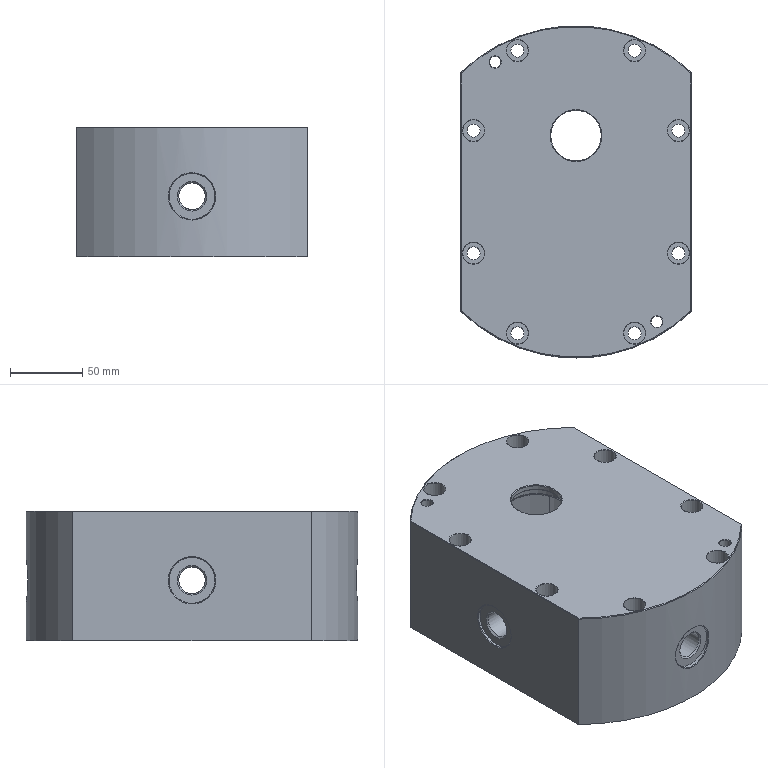NC program | NX | posted with a generic post | part box 160 x 230 x 90 mm
Lines 8806 to 9223 of 9223:
(HOLE_MILLING_COPY_COPY_COPY_COPY , TOOL : D12)
N17568 T12 M6
N17570 G54
N17572 G17 G0 G90 X43.9 Y6.945 B0. C0. S3000 M3
N17574 G43 Z30. H12
N17576 Z-77.5
N17578 G94 G3 X39. Y16.4 R5.997 F1500.
N17580 X39. Y16.4 Z-77.72 I0. J-16.4
N17582 X39. Y16.4 Z-77.94 I0. J-16.4
N17584 X39. Y16.4 Z-78.16 I0. J-16.4
N17586 X39. Y16.4 Z-78.38 I0. J-16.4
N17588 X39. Y16.4 Z-78.6 I0. J-16.4
N17590 X39. Y16.4 Z-78.82 I0. J-16.4
N17592 X39. Y16.4 Z-79.04 I0. J-16.4
N17594 X39. Y16.4 Z-79.26 I0. J-16.4
N17596 X39. Y16.4 Z-79.48 I0. J-16.4
N17598 X39. Y16.4 Z-79.7 I0. J-16.4
N17600 X39. Y16.4 Z-79.92 I0. J-16.4
N17602 X39. Y16.4 Z-80.14 I0. J-16.4
N17604 X39. Y16.4 Z-80.36 I0. J-16.4
N17606 X39. Y16.4 Z-80.58 I0. J-16.4
N17608 X39. Y16.4 Z-80.8 I0. J-16.4
N17610 X39. Y16.4 Z-81.02 I0. J-16.4
N17612 X39. Y16.4 Z-81.24 I0. J-16.4
N17614 X39. Y16.4 Z-81.46 I0. J-16.4
N17616 X39. Y16.4 Z-81.68 I0. J-16.4
N17618 X39. Y16.4 Z-81.9 I0. J-16.4
N17620 X39. Y16.4 Z-82.12 I0. J-16.4
N17622 X39. Y16.4 Z-82.34 I0. J-16.4
N17624 X39. Y16.4 Z-82.56 I0. J-16.4
N17626 X39. Y16.4 Z-82.78 I0. J-16.4
N17628 X39. Y16.4 Z-83. I0. J-16.4
N17630 X39. Y16.4 Z-83.22 I0. J-16.4
N17632 X39. Y16.4 Z-83.44 I0. J-16.4
N17634 X39. Y16.4 Z-83.66 I0. J-16.4
N17636 X39. Y16.4 Z-83.88 I0. J-16.4
N17638 X39. Y16.4 Z-84.1 I0. J-16.4
N17640 X39. Y16.4 Z-84.32 I0. J-16.4
N17642 X39. Y16.4 Z-84.54 I0. J-16.4
N17644 X39. Y16.4 Z-84.76 I0. J-16.4
N17646 X39. Y16.4 Z-84.98 I0. J-16.4
N17648 X39. Y16.4 Z-85.2 I0. J-16.4
N17650 X39. Y16.4 Z-85.42 I0. J-16.4
N17652 X39. Y16.4 Z-85.64 I0. J-16.4
N17654 X39. Y16.4 Z-85.86 I0. J-16.4
N17656 X51.394 Y-10.74 Z-86. R-16.4
N17658 X49.74 Y12.394 R16.4
N17660 X51.394 Y-10.74 R-16.4
N17662 X47.458 Y-0.845 R5.997
N17664 G0 Z30.
(FLOOR_WALL_1_COPY , TOOL : D12)
N17666 X-67.913 Y-48.287 S4000
N17668 Z-6.738
N17670 G1 Z-9.738 F500.
N17672 X-66.116 Y-51.4
N17674 G3 X-65.077 Y-52. R1.2
N17676 G1 X65.077 F1000.
N17678 G3 X72.586 Y-47.962 R9.
N17680 X72.586 Y47.962 R87.
N17682 X65.077 Y52. R9.
N17684 G1 X-65.077
N17686 G3 X-72.586 Y47.962 R9.
N17688 X-72.586 Y-47.962 R87.
N17690 X-65.077 Y-52. R9.
N17692 X-64.038 Y-51.4 R1.2
N17694 G1 X-62.652 Y-49.
N17696 Z-6.738
N17698 G0 X-67.913 Y-48.287 Z-16.475
N17700 G1 Z-19.475 F500.
N17702 X-66.116 Y-51.4
N17704 G3 X-65.077 Y-52. R1.2
N17706 G1 X65.077 F1000.
N17708 G3 X72.586 Y-47.962 R9.
N17710 X72.586 Y47.962 R87.
N17712 X65.077 Y52. R9.
N17714 G1 X-65.077
N17716 G3 X-72.586 Y47.962 R9.
N17718 X-72.586 Y-47.962 R87.
N17720 X-65.077 Y-52. R9.
N17722 X-64.038 Y-51.4 R1.2
N17724 G1 X-62.652 Y-49.
N17726 Z-16.475
N17728 G0 X-67.913 Y-48.287 Z-26.213
N17730 G1 Z-29.213 F500.
N17732 X-66.116 Y-51.4
N17734 G3 X-65.077 Y-52. R1.2
N17736 G1 X65.077 F1000.
N17738 G3 X72.586 Y-47.962 R9.
N17740 X72.586 Y47.962 R87.
N17742 X65.077 Y52. R9.
N17744 G1 X-65.077
N17746 G3 X-72.586 Y47.962 R9.
N17748 X-72.586 Y-47.962 R87.
N17750 X-65.077 Y-52. R9.
N17752 X-64.038 Y-51.4 R1.2
N17754 G1 X-62.652 Y-49.
N17756 Z-26.213
N17758 G0 X-67.913 Y-48.287 Z-35.95
N17760 G1 Z-38.95 F500.
N17762 X-66.116 Y-51.4
N17764 G3 X-65.077 Y-52. R1.2
N17766 G1 X65.077 F1000.
N17768 G3 X72.586 Y-47.962 R9.
N17770 X72.586 Y47.962 R87.
N17772 X65.077 Y52. R9.
N17774 G1 X-65.077
N17776 G3 X-72.586 Y47.962 R9.
N17778 X-72.586 Y-47.962 R87.
N17780 X-65.077 Y-52. R9.
N17782 X-64.038 Y-51.4 R1.2
N17784 G1 X-62.652 Y-49.
N17786 Z-35.95
N17788 G0 X-67.913 Y-48.287 Z-45.688
N17790 G1 Z-48.688 F500.
N17792 X-66.116 Y-51.4
N17794 G3 X-65.077 Y-52. R1.2
N17796 G1 X65.077 F1000.
N17798 G3 X72.586 Y-47.962 R9.
N17800 X72.586 Y47.962 R87.
N17802 X65.077 Y52. R9.
N17804 G1 X-65.077
N17806 G3 X-72.586 Y47.962 R9.
N17808 X-72.586 Y-47.962 R87.
N17810 X-65.077 Y-52. R9.
N17812 X-64.038 Y-51.4 R1.2
N17814 G1 X-62.652 Y-49.
N17816 Z-45.688
N17818 G0 X-67.913 Y-48.287 Z-55.425
N17820 G1 Z-58.425 F500.
N17822 X-66.116 Y-51.4
N17824 G3 X-65.077 Y-52. R1.2
N17826 G1 X65.077 F1000.
N17828 G3 X72.586 Y-47.962 R9.
N17830 X72.586 Y47.962 R87.
N17832 X65.077 Y52. R9.
N17834 G1 X-65.077
N17836 G3 X-72.586 Y47.962 R9.
N17838 X-72.586 Y-47.962 R87.
N17840 X-65.077 Y-52. R9.
N17842 X-64.038 Y-51.4 R1.2
N17844 G1 X-62.652 Y-49.
N17846 Z-55.425
N17848 G0 X-67.913 Y-48.287 Z-65.163
N17850 G1 Z-68.163 F500.
N17852 X-66.116 Y-51.4
N17854 G3 X-65.077 Y-52. R1.2
N17856 G1 X65.077 F1000.
N17858 G3 X72.586 Y-47.962 R9.
N17860 X72.586 Y47.962 R87.
N17862 X65.077 Y52. R9.
N17864 G1 X-65.077
N17866 G3 X-72.586 Y47.962 R9.
N17868 X-72.586 Y-47.962 R87.
N17870 X-65.077 Y-52. R9.
N17872 X-64.038 Y-51.4 R1.2
N17874 G1 X-62.652 Y-49.
N17876 Z-65.163
N17878 G0 X-67.913 Y-48.287 Z-74.9
N17880 G1 Z-77.9 F500.
N17882 X-66.116 Y-51.4
N17884 G3 X-65.077 Y-52. R1.2
N17886 G1 X65.077 F1000.
N17888 G3 X72.586 Y-47.962 R9.
N17890 X72.586 Y47.962 R87.
N17892 X65.077 Y52. R9.
N17894 G1 X-65.077
N17896 G3 X-72.586 Y47.962 R9.
N17898 X-72.586 Y-47.962 R87.
N17900 X-65.077 Y-52. R9.
N17902 X-64.038 Y-51.4 R1.2
N17904 G1 X-62.652 Y-49.
N17906 Z-74.9
N17908 G0 Z30.
(FLOOR_WALL_1_COPY_COPY , TOOL : D12)
N17910 X-64.167 Y50.799
N17912 Z-75.
N17914 G1 Z-78. F500.
N17916 G3 X-65.206 Y51.399 R1.2
N17918 G1 X65.206 F1000.
N17920 G2 X72.085 Y47.631 R8.4
N17922 X73.332 Y45.688 R86.4
N17924 G1 X-73.332
N17926 G3 X-76.595 Y39.977 R86.4
N17928 G1 X76.595
N17930 G2 X79.315 Y34.266 R86.4
N17932 G1 X-79.315
N17934 G3 X-81.545 Y28.555 R86.4
N17936 G1 X81.545
N17938 G2 X83.325 Y22.844 R86.4
N17940 G1 X-83.325
N17942 G3 X-84.684 Y17.133 R86.4
N17944 G1 X84.684
N17946 G2 X85.642 Y11.422 R86.4
N17948 G1 X-85.642
N17950 G3 X-86.211 Y5.711 R86.4
N17952 G1 X86.211
N17954 G2 X86.4 Y0. R86.4
N17956 G1 X-86.4
N17958 G3 X-86.211 Y-5.712 R86.4
N17960 G1 X86.211
N17962 G2 X85.642 Y-11.423 R86.4
N17964 G1 X-85.642
N17966 G3 X-84.684 Y-17.134 R86.4
N17968 G1 X84.684
N17970 G2 X83.325 Y-22.845 R86.4
N17972 G1 X-83.325
N17974 G3 X-81.545 Y-28.556 R86.4
N17976 G1 X81.545
N17978 G2 X79.314 Y-34.267 R86.4
N17980 G1 X-79.314
N17982 G3 X-76.595 Y-39.978 R86.4
N17984 G1 X76.595
N17986 G2 X73.331 Y-45.689 R86.4
N17988 G1 X-73.331
N17990 G3 X-72.085 Y-47.631 R86.4
N17992 X-65.09 Y-51.4 R8.4
N17994 G1 X65.09
N17996 G3 X66.13 Y-50.8 R1.2
N17998 G1 X64.051 Y-51.402
N18000 G3 X65.091 Y-52. R1.2 F500.
N18002 X72.586 Y-47.962 R9. F1000.
N18004 X72.586 Y47.962 R87.
N18006 X65.077 Y52. R9.
N18008 G1 X-65.077
N18010 G3 X-72.586 Y47.962 R9.
N18012 X-72.586 Y-47.962 R87.
N18014 X-65.077 Y-52. R9.
N18016 G1 X65.091
N18018 G3 X66.13 Y-51.398 R1.2
N18020 G1 X67.922 Y-48.283
N18022 Z-75.
N18024 G0 Z30.
N18026 M5
(PLANAR_MILL_COPY_COPY_COPY , TOOL : D6A45)
N18028 T07 M6
N18030 G54
N18032 G17 G0 G90 X-43.266 Y-73.843 B0. C0. S7500 M3
N18034 G43 Z30. H7
N18036 Z1.5
N18038 G94 G1 Z-1.5 F1250.
N18040 G3 X-42.5 Y-74.2 R1.
N18042 X-39.3 Y-71. R3.2
N18044 X-42.5 Y-74.2 R-3.2
N18046 X-41.734 Y-73.843 R1.
N18048 G1 Z1.5
N18050 G0 Z30.
N18052 X-100.774 Y-39.798
N18054 Z1.5
N18056 G1 Z-1.5
N18058 G3 X-101.131 Y-40.564 R1.
N18060 X-97.931 Y-43.764 R3.2
N18062 X-101.131 Y-40.564 R-3.2
N18064 X-100.774 Y-41.33 R1.
N18066 G1 Z1.5
N18068 G0 Z30.
N18070 Y41.33
N18072 Z1.5
N18074 G1 Z-1.5
N18076 G3 X-101.131 Y40.564 R1.
N18078 X-97.931 Y37.364 R3.2
N18080 X-101.131 Y40.564 R-3.2
N18082 X-100.774 Y39.798 R1.
N18084 G1 Z1.5
N18086 G0 Z30.
N18088 X-92.343 Y56.766
N18090 Z1.5
N18092 G1 Z-1.5
N18094 G3 X-92.7 Y56. R1.
N18096 X-90. Y53.3 R2.7
N18098 X-92.7 Y56. R-2.7
N18100 X-92.343 Y55.234 R1.
N18102 G1 Z1.5
N18104 G0 Z30.
N18106 X-41.734 Y73.843
N18108 Z1.5
N18110 G1 Z-1.5
N18112 G3 X-42.5 Y74.2 R1.
N18114 X-45.7 Y71. R3.2
N18116 X-42.5 Y74.2 R-3.2
N18118 X-43.266 Y73.843 R1.
N18120 G1 Z1.5
N18122 G0 Z30.
N18124 X-0.766 Y62.657
N18126 Z1.5
N18128 G1 Z-1.5
N18130 G3 X0. Y62.3 R1.
N18132 G1 X65.077
N18134 G2 X81.179 Y53.64 R19.3
N18136 X81.179 Y-53.64 R97.3
N18138 X65.077 Y-62.3 R19.3
N18140 G1 X-65.077
N18142 G2 X-81.179 Y-53.64 R19.3
N18144 X-81.179 Y53.64 R97.3
N18146 X-65.077 Y62.3 R19.3
N18148 G1 X0.
N18150 G3 X0.766 Y62.657 R1.
N18152 G1 Z1.5
N18154 G0 Z30.
N18156 Y62.343
N18158 Z1.5
N18160 G1 Z-1.5
N18162 G3 X0. Y62.7 R1.
N18164 G1 X-65.077
N18166 G3 X-81.513 Y53.86 R19.7
N18168 X-81.513 Y-53.86 R97.7
N18170 X-65.077 Y-62.7 R19.7
N18172 G1 X65.077
N18174 G3 X81.513 Y-53.86 R19.7
N18176 X81.513 Y53.86 R97.7
N18178 X65.077 Y62.7 R19.7
N18180 G1 X0.
N18182 G3 X-0.766 Y62.343 R1.
N18184 G1 Z1.5
N18186 G0 Z30.
N18188 Y81.657
N18190 Z1.5
N18192 G1 Z-1.5
N18194 G3 X0. Y81.3 R1.
N18196 G1 X82.614
N18198 G2 X83.547 Y80.904 R1.3
N18200 X83.547 Y-80.904 R116.3
N18202 X82.614 Y-81.3 R1.3
N18204 G1 X-82.614
N18206 G2 X-83.547 Y-80.904 R1.3
N18208 X-83.547 Y80.904 R116.3
N18210 X-82.614 Y81.3 R1.3
N18212 G1 X0.
N18214 G3 X0.766 Y81.657 R1.
N18216 G1 Z1.5
N18218 G0 Z30.
N18220 Y56.343
N18222 Z1.5
N18224 G1 Z-1.5
N18226 G3 X0. Y56.7 R1.
N18228 G1 X-65.077
N18230 G3 X-76.507 Y50.553 R13.7
N18232 X-76.507 Y-50.553 R91.7
N18234 X-65.077 Y-56.7 R13.7
N18236 G1 X65.077
N18238 G3 X76.507 Y-50.553 R13.7
N18240 X76.507 Y50.553 R91.7
N18242 X65.077 Y56.7 R13.7
N18244 G1 X0.
N18246 G3 X-0.766 Y56.343 R1.
N18248 G1 Z1.5
N18250 G0 Z30.
N18252 X41.734 Y-73.843
N18254 Z1.5
N18256 G1 Z-1.5
N18258 G3 X42.5 Y-74.2 R1.
N18260 X45.7 Y-71. R3.2
N18262 X42.5 Y-74.2 R-3.2
N18264 X43.266 Y-73.843 R1.
N18266 G1 Z1.5
N18268 G0 Z30.
N18270 X89.234 Y-58.343
N18272 Z1.5
N18274 G1 Z-1.5
N18276 G3 X90. Y-58.7 R1.
N18278 X92.7 Y-56. R2.7
N18280 X90. Y-58.7 R-2.7
N18282 X90.766 Y-58.343 R1.
N18284 G1 Z1.5
N18286 G0 Z30.
N18288 X100.774 Y-41.33
N18290 Z1.5
N18292 G1 Z-1.5
N18294 G3 X101.131 Y-40.564 R1.
N18296 X97.931 Y-37.364 R3.2
N18298 X101.131 Y-40.564 R-3.2
N18300 X100.774 Y-39.798 R1.
N18302 G1 Z1.5
N18304 G0 Z30.
N18306 Y39.798
N18308 Z1.5
N18310 G1 Z-1.5
N18312 G3 X101.131 Y40.564 R1.
N18314 X97.931 Y43.764 R3.2
N18316 X101.131 Y40.564 R-3.2
N18318 X100.774 Y41.33 R1.
N18320 G1 Z1.5
N18322 G0 Z30.
N18324 X43.266 Y73.843
N18326 Z1.5
N18328 G1 Z-1.5
N18330 G3 X42.5 Y74.2 R1.
N18332 X39.3 Y71. R3.2
N18334 X42.5 Y74.2 R-3.2
N18336 X41.734 Y73.843 R1.
N18338 G1 Z1.5
N18340 G0 Z30.
N18342 M5
(CUTTER_COMP_12 , TOOL : D12)
N18344 T12 M6
N18346 G54
N18348 G17 G0 G90 X42.192 Y12.911 B0. C0. S4000 M3
N18350 G43 Z30. H12
N18352 Z-86.
N18354 G41 G94 G1 X42.216 Y13.008 F1000. D12
N18356 G3 X39. Y16.45 R3.223
N18358 X22.55 Y0. R16.45
N18360 X39. Y16.45 R-16.45
N18362 X35.784 Y13.008 R3.223
N18364 G40
N18366 G1 X35.808 Y12.911
N18368 G0 Z30.
N18370 M5
N18372 M2